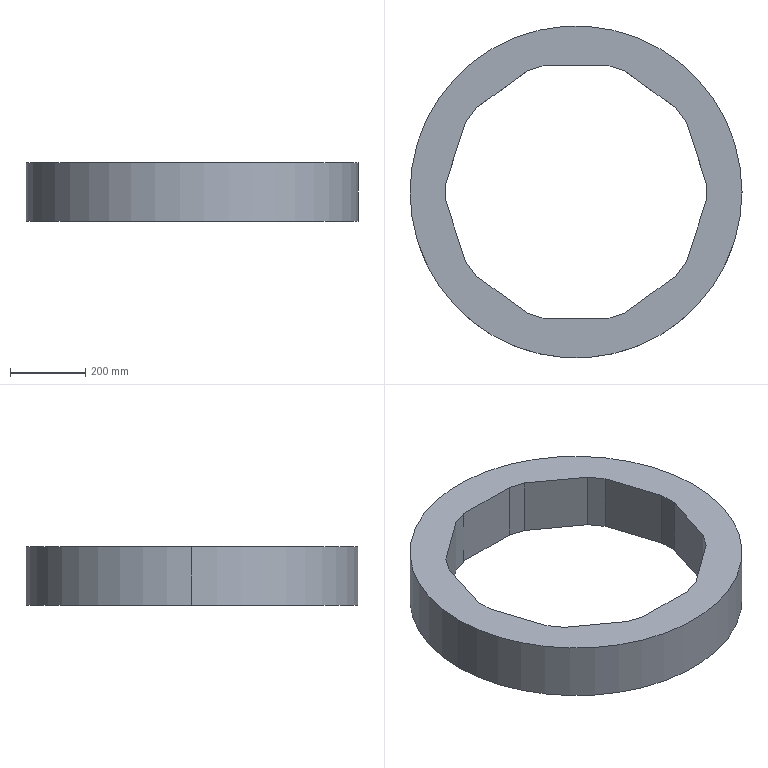Part | SolidWorks | features Extrusion 1 | 1 solid | 24 faces | box 884 x 884 x 155 mm | volume 38209027 mm3 | plane 22 | cylinder 2 | commonest cylinder face diameters 884 x2
STEP:
#1=CARTESIAN_POINT('',(442.,0.,77.5));
#2=VERTEX_POINT('',#1);
#3=CARTESIAN_POINT('',(-442.,0.,77.5));
#4=VERTEX_POINT('',#3);
#5=CARTESIAN_POINT('',(0.,0.,77.5));
#6=DIRECTION('',(0.,0.,1.));
#7=DIRECTION('',(1.,0.,0.));
#8=AXIS2_PLACEMENT_3D('',#5,#6,#7);
#9=CIRCLE('',#8,442.);
#10=EDGE_CURVE('',#2,#4,#9,.T.);
#11=ORIENTED_EDGE('',*,*,#10,.F.);
#12=CARTESIAN_POINT('',(442.,0.,-77.5));
#13=VERTEX_POINT('',#12);
#14=CARTESIAN_POINT('',(442.,0.,77.5));
#15=DIRECTION('',(0.,0.,-1.));
#16=VECTOR('',#15,1000.);
#17=LINE('',#14,#16);
#18=EDGE_CURVE('',#2,#13,#17,.T.);
#19=ORIENTED_EDGE('',*,*,#18,.T.);
#20=CARTESIAN_POINT('',(-442.,0.,-77.5));
#21=VERTEX_POINT('',#20);
#22=CARTESIAN_POINT('',(0.,0.,-77.5));
#23=DIRECTION('',(0.,0.,1.));
#24=DIRECTION('',(1.,0.,0.));
#25=AXIS2_PLACEMENT_3D('',#22,#23,#24);
#26=CIRCLE('',#25,442.);
#27=EDGE_CURVE('',#13,#21,#26,.T.);
#28=ORIENTED_EDGE('',*,*,#27,.T.);
#29=CARTESIAN_POINT('',(-442.,0.,77.5));
#30=DIRECTION('',(0.,0.,-1.));
#31=VECTOR('',#30,1000.);
#32=LINE('',#29,#31);
#33=EDGE_CURVE('',#4,#21,#32,.T.);
#34=ORIENTED_EDGE('',*,*,#33,.F.);
#35=EDGE_LOOP('',(#11,#19,#28,#34));
#36=FACE_OUTER_BOUND('',#35,.T.);
#37=CARTESIAN_POINT('',(0.,0.,77.5));
#38=DIRECTION('',(0.,0.,-1.));
#39=DIRECTION('',(-1.,0.,0.));
#40=AXIS2_PLACEMENT_3D('',#37,#38,#39);
#41=CYLINDRICAL_SURFACE('',#40,442.);
#42=ADVANCED_FACE('',(#36),#41,.T.);
#43=CARTESIAN_POINT('',(0.,0.,77.5));
#44=DIRECTION('',(0.,0.,1.));
#45=DIRECTION('',(1.,0.,0.));
#46=AXIS2_PLACEMENT_3D('',#43,#44,#45);
#47=CIRCLE('',#46,442.);
#48=EDGE_CURVE('',#4,#2,#47,.T.);
#49=ORIENTED_EDGE('',*,*,#48,.T.);
#50=ORIENTED_EDGE('',*,*,#10,.T.);
#51=EDGE_LOOP('',(#49,#50));
#52=FACE_OUTER_BOUND('',#51,.T.);
#53=CARTESIAN_POINT('',(346.772,-23.299,77.5));
#54=VERTEX_POINT('',#53);
#55=CARTESIAN_POINT('',(346.772,23.299,77.5));
#56=VERTEX_POINT('',#55);
#57=CARTESIAN_POINT('',(346.772,-23.299,77.5));
#58=DIRECTION('',(0.,1.,0.));
#59=VECTOR('',#58,1000.);
#60=LINE('',#57,#59);
#61=EDGE_CURVE('',#54,#56,#60,.T.);
#62=ORIENTED_EDGE('',*,*,#61,.F.);
#63=CARTESIAN_POINT('',(294.24,-184.979,77.5));
#64=VERTEX_POINT('',#63);
#65=CARTESIAN_POINT('',(346.772,-23.299,77.5));
#66=DIRECTION('',(0.309,0.9511,0.));
#67=VECTOR('',#66,1000.);
#68=LINE('',#65,#67);
#69=EDGE_CURVE('',#64,#54,#68,.T.);
#70=ORIENTED_EDGE('',*,*,#69,.F.);
#71=CARTESIAN_POINT('',(266.85,-222.677,77.5));
#72=VERTEX_POINT('',#71);
#73=CARTESIAN_POINT('',(294.24,-184.979,77.5));
#74=DIRECTION('',(0.5878,0.809,0.));
#75=VECTOR('',#74,1000.);
#76=LINE('',#73,#75);
#77=EDGE_CURVE('',#72,#64,#76,.T.);
#78=ORIENTED_EDGE('',*,*,#77,.F.);
#79=CARTESIAN_POINT('',(129.317,-322.6,77.5));
#80=VERTEX_POINT('',#79);
#81=CARTESIAN_POINT('',(266.85,-222.677,77.5));
#82=DIRECTION('',(0.809,0.5878,0.));
#83=VECTOR('',#82,1000.);
#84=LINE('',#81,#83);
#85=EDGE_CURVE('',#80,#72,#84,.T.);
#86=ORIENTED_EDGE('',*,*,#85,.F.);
#87=CARTESIAN_POINT('',(85.,-337.,77.5));
#88=VERTEX_POINT('',#87);
#89=CARTESIAN_POINT('',(85.,-337.,77.5));
#90=DIRECTION('',(0.9511,0.309,0.));
#91=VECTOR('',#90,1000.);
#92=LINE('',#89,#91);
#93=EDGE_CURVE('',#88,#80,#92,.T.);
#94=ORIENTED_EDGE('',*,*,#93,.F.);
#95=CARTESIAN_POINT('',(-85.,-337.,77.5));
#96=VERTEX_POINT('',#95);
#97=CARTESIAN_POINT('',(85.,-337.,77.5));
#98=DIRECTION('',(1.,0.,0.));
#99=VECTOR('',#98,1000.);
#100=LINE('',#97,#99);
#101=EDGE_CURVE('',#96,#88,#100,.T.);
#102=ORIENTED_EDGE('',*,*,#101,.F.);
#103=CARTESIAN_POINT('',(-129.317,-322.6,77.5));
#104=VERTEX_POINT('',#103);
#105=CARTESIAN_POINT('',(-129.317,-322.6,77.5));
#106=DIRECTION('',(0.9511,-0.309,0.));
#107=VECTOR('',#106,1000.);
#108=LINE('',#105,#107);
#109=EDGE_CURVE('',#104,#96,#108,.T.);
#110=ORIENTED_EDGE('',*,*,#109,.F.);
#111=CARTESIAN_POINT('',(-266.85,-222.677,77.5));
#112=VERTEX_POINT('',#111);
#113=CARTESIAN_POINT('',(-129.317,-322.6,77.5));
#114=DIRECTION('',(0.809,-0.5878,0.));
#115=VECTOR('',#114,1000.);
#116=LINE('',#113,#115);
#117=EDGE_CURVE('',#112,#104,#116,.T.);
#118=ORIENTED_EDGE('',*,*,#117,.F.);
#119=CARTESIAN_POINT('',(-294.24,-184.979,77.5));
#120=VERTEX_POINT('',#119);
#121=CARTESIAN_POINT('',(-294.24,-184.979,77.5));
#122=DIRECTION('',(0.5878,-0.809,0.));
#123=VECTOR('',#122,1000.);
#124=LINE('',#121,#123);
#125=EDGE_CURVE('',#120,#112,#124,.T.);
#126=ORIENTED_EDGE('',*,*,#125,.F.);
#127=CARTESIAN_POINT('',(-346.772,-23.299,77.5));
#128=VERTEX_POINT('',#127);
#129=CARTESIAN_POINT('',(-294.24,-184.979,77.5));
#130=DIRECTION('',(0.309,-0.9511,0.));
#131=VECTOR('',#130,1000.);
#132=LINE('',#129,#131);
#133=EDGE_CURVE('',#128,#120,#132,.T.);
#134=ORIENTED_EDGE('',*,*,#133,.F.);
#135=CARTESIAN_POINT('',(-346.772,23.299,77.5));
#136=VERTEX_POINT('',#135);
#137=CARTESIAN_POINT('',(-346.772,23.299,77.5));
#138=DIRECTION('',(0.,-1.,0.));
#139=VECTOR('',#138,1000.);
#140=LINE('',#137,#139);
#141=EDGE_CURVE('',#136,#128,#140,.T.);
#142=ORIENTED_EDGE('',*,*,#141,.F.);
#143=CARTESIAN_POINT('',(-294.24,184.979,77.5));
#144=VERTEX_POINT('',#143);
#145=CARTESIAN_POINT('',(-346.772,23.299,77.5));
#146=DIRECTION('',(-0.309,-0.9511,0.));
#147=VECTOR('',#146,1000.);
#148=LINE('',#145,#147);
#149=EDGE_CURVE('',#144,#136,#148,.T.);
#150=ORIENTED_EDGE('',*,*,#149,.F.);
#151=CARTESIAN_POINT('',(-266.85,222.677,77.5));
#152=VERTEX_POINT('',#151);
#153=CARTESIAN_POINT('',(-266.85,222.677,77.5));
#154=DIRECTION('',(-0.5878,-0.809,0.));
#155=VECTOR('',#154,1000.);
#156=LINE('',#153,#155);
#157=EDGE_CURVE('',#152,#144,#156,.T.);
#158=ORIENTED_EDGE('',*,*,#157,.F.);
#159=CARTESIAN_POINT('',(-129.317,322.6,77.5));
#160=VERTEX_POINT('',#159);
#161=CARTESIAN_POINT('',(-266.85,222.677,77.5));
#162=DIRECTION('',(-0.809,-0.5878,0.));
#163=VECTOR('',#162,1000.);
#164=LINE('',#161,#163);
#165=EDGE_CURVE('',#160,#152,#164,.T.);
#166=ORIENTED_EDGE('',*,*,#165,.F.);
#167=CARTESIAN_POINT('',(-85.,337.,77.5));
#168=VERTEX_POINT('',#167);
#169=CARTESIAN_POINT('',(-85.,337.,77.5));
#170=DIRECTION('',(-0.9511,-0.309,0.));
#171=VECTOR('',#170,1000.);
#172=LINE('',#169,#171);
#173=EDGE_CURVE('',#168,#160,#172,.T.);
#174=ORIENTED_EDGE('',*,*,#173,.F.);
#175=CARTESIAN_POINT('',(85.,337.,77.5));
#176=VERTEX_POINT('',#175);
#177=CARTESIAN_POINT('',(-85.,337.,77.5));
#178=DIRECTION('',(-1.,0.,0.));
#179=VECTOR('',#178,1000.);
#180=LINE('',#177,#179);
#181=EDGE_CURVE('',#176,#168,#180,.T.);
#182=ORIENTED_EDGE('',*,*,#181,.F.);
#183=CARTESIAN_POINT('',(129.317,322.6,77.5));
#184=VERTEX_POINT('',#183);
#185=CARTESIAN_POINT('',(129.317,322.6,77.5));
#186=DIRECTION('',(-0.9511,0.309,0.));
#187=VECTOR('',#186,1000.);
#188=LINE('',#185,#187);
#189=EDGE_CURVE('',#184,#176,#188,.T.);
#190=ORIENTED_EDGE('',*,*,#189,.F.);
#191=CARTESIAN_POINT('',(266.85,222.677,77.5));
#192=VERTEX_POINT('',#191);
#193=CARTESIAN_POINT('',(129.317,322.6,77.5));
#194=DIRECTION('',(-0.809,0.5878,0.));
#195=VECTOR('',#194,1000.);
#196=LINE('',#193,#195);
#197=EDGE_CURVE('',#192,#184,#196,.T.);
#198=ORIENTED_EDGE('',*,*,#197,.F.);
#199=CARTESIAN_POINT('',(294.24,184.979,77.5));
#200=VERTEX_POINT('',#199);
#201=CARTESIAN_POINT('',(294.24,184.979,77.5));
#202=DIRECTION('',(-0.5878,0.809,0.));
#203=VECTOR('',#202,1000.);
#204=LINE('',#201,#203);
#205=EDGE_CURVE('',#200,#192,#204,.T.);
#206=ORIENTED_EDGE('',*,*,#205,.F.);
#207=CARTESIAN_POINT('',(294.24,184.979,77.5));
#208=DIRECTION('',(-0.309,0.9511,0.));
#209=VECTOR('',#208,1000.);
#210=LINE('',#207,#209);
#211=EDGE_CURVE('',#56,#200,#210,.T.);
#212=ORIENTED_EDGE('',*,*,#211,.F.);
#213=EDGE_LOOP('',(#62,#70,#78,#86,#94,#102,#110,#118,#126,#134,#142,#150,#158,#166,#174,#182,#190,#198,#206,#212));
#214=FACE_BOUND('',#213,.T.);
#215=CARTESIAN_POINT('',(0.,0.,77.5));
#216=DIRECTION('',(0.,0.,1.));
#217=DIRECTION('',(1.,0.,0.));
#218=AXIS2_PLACEMENT_3D('',#215,#216,#217);
#219=PLANE('',#218);
#220=ADVANCED_FACE('',(#52,#214),#219,.T.);
#221=CARTESIAN_POINT('',(0.,0.,-77.5));
#222=DIRECTION('',(0.,0.,1.));
#223=DIRECTION('',(1.,0.,0.));
#224=AXIS2_PLACEMENT_3D('',#221,#222,#223);
#225=CIRCLE('',#224,442.);
#226=EDGE_CURVE('',#21,#13,#225,.T.);
#227=ORIENTED_EDGE('',*,*,#226,.F.);
#228=ORIENTED_EDGE('',*,*,#27,.F.);
#229=EDGE_LOOP('',(#227,#228));
#230=FACE_OUTER_BOUND('',#229,.T.);
#231=CARTESIAN_POINT('',(294.24,-184.979,-77.5));
#232=VERTEX_POINT('',#231);
#233=CARTESIAN_POINT('',(346.772,-23.299,-77.5));
#234=VERTEX_POINT('',#233);
#235=CARTESIAN_POINT('',(346.772,-23.299,-77.5));
#236=DIRECTION('',(0.309,0.9511,0.));
#237=VECTOR('',#236,1000.);
#238=LINE('',#235,#237);
#239=EDGE_CURVE('',#232,#234,#238,.T.);
#240=ORIENTED_EDGE('',*,*,#239,.T.);
#241=CARTESIAN_POINT('',(346.772,23.299,-77.5));
#242=VERTEX_POINT('',#241);
#243=CARTESIAN_POINT('',(346.772,-23.299,-77.5));
#244=DIRECTION('',(0.,1.,0.));
#245=VECTOR('',#244,1000.);
#246=LINE('',#243,#245);
#247=EDGE_CURVE('',#234,#242,#246,.T.);
#248=ORIENTED_EDGE('',*,*,#247,.T.);
#249=CARTESIAN_POINT('',(294.24,184.979,-77.5));
#250=VERTEX_POINT('',#249);
#251=CARTESIAN_POINT('',(294.24,184.979,-77.5));
#252=DIRECTION('',(-0.309,0.9511,0.));
#253=VECTOR('',#252,1000.);
#254=LINE('',#251,#253);
#255=EDGE_CURVE('',#242,#250,#254,.T.);
#256=ORIENTED_EDGE('',*,*,#255,.T.);
#257=CARTESIAN_POINT('',(266.85,222.677,-77.5));
#258=VERTEX_POINT('',#257);
#259=CARTESIAN_POINT('',(294.24,184.979,-77.5));
#260=DIRECTION('',(-0.5878,0.809,0.));
#261=VECTOR('',#260,1000.);
#262=LINE('',#259,#261);
#263=EDGE_CURVE('',#250,#258,#262,.T.);
#264=ORIENTED_EDGE('',*,*,#263,.T.);
#265=CARTESIAN_POINT('',(129.317,322.6,-77.5));
#266=VERTEX_POINT('',#265);
#267=CARTESIAN_POINT('',(129.317,322.6,-77.5));
#268=DIRECTION('',(-0.809,0.5878,0.));
#269=VECTOR('',#268,1000.);
#270=LINE('',#267,#269);
#271=EDGE_CURVE('',#258,#266,#270,.T.);
#272=ORIENTED_EDGE('',*,*,#271,.T.);
#273=CARTESIAN_POINT('',(85.,337.,-77.5));
#274=VERTEX_POINT('',#273);
#275=CARTESIAN_POINT('',(129.317,322.6,-77.5));
#276=DIRECTION('',(-0.9511,0.309,0.));
#277=VECTOR('',#276,1000.);
#278=LINE('',#275,#277);
#279=EDGE_CURVE('',#266,#274,#278,.T.);
#280=ORIENTED_EDGE('',*,*,#279,.T.);
#281=CARTESIAN_POINT('',(-85.,337.,-77.5));
#282=VERTEX_POINT('',#281);
#283=CARTESIAN_POINT('',(-85.,337.,-77.5));
#284=DIRECTION('',(-1.,0.,0.));
#285=VECTOR('',#284,1000.);
#286=LINE('',#283,#285);
#287=EDGE_CURVE('',#274,#282,#286,.T.);
#288=ORIENTED_EDGE('',*,*,#287,.T.);
#289=CARTESIAN_POINT('',(-129.317,322.6,-77.5));
#290=VERTEX_POINT('',#289);
#291=CARTESIAN_POINT('',(-85.,337.,-77.5));
#292=DIRECTION('',(-0.9511,-0.309,0.));
#293=VECTOR('',#292,1000.);
#294=LINE('',#291,#293);
#295=EDGE_CURVE('',#282,#290,#294,.T.);
#296=ORIENTED_EDGE('',*,*,#295,.T.);
#297=CARTESIAN_POINT('',(-266.85,222.677,-77.5));
#298=VERTEX_POINT('',#297);
#299=CARTESIAN_POINT('',(-266.85,222.677,-77.5));
#300=DIRECTION('',(-0.809,-0.5878,0.));
#301=VECTOR('',#300,1000.);
#302=LINE('',#299,#301);
#303=EDGE_CURVE('',#290,#298,#302,.T.);
#304=ORIENTED_EDGE('',*,*,#303,.T.);
#305=CARTESIAN_POINT('',(-294.24,184.979,-77.5));
#306=VERTEX_POINT('',#305);
#307=CARTESIAN_POINT('',(-266.85,222.677,-77.5));
#308=DIRECTION('',(-0.5878,-0.809,0.));
#309=VECTOR('',#308,1000.);
#310=LINE('',#307,#309);
#311=EDGE_CURVE('',#298,#306,#310,.T.);
#312=ORIENTED_EDGE('',*,*,#311,.T.);
#313=CARTESIAN_POINT('',(-346.772,23.299,-77.5));
#314=VERTEX_POINT('',#313);
#315=CARTESIAN_POINT('',(-346.772,23.299,-77.5));
#316=DIRECTION('',(-0.309,-0.9511,0.));
#317=VECTOR('',#316,1000.);
#318=LINE('',#315,#317);
#319=EDGE_CURVE('',#306,#314,#318,.T.);
#320=ORIENTED_EDGE('',*,*,#319,.T.);
#321=CARTESIAN_POINT('',(-346.772,-23.299,-77.5));
#322=VERTEX_POINT('',#321);
#323=CARTESIAN_POINT('',(-346.772,23.299,-77.5));
#324=DIRECTION('',(0.,-1.,0.));
#325=VECTOR('',#324,1000.);
#326=LINE('',#323,#325);
#327=EDGE_CURVE('',#314,#322,#326,.T.);
#328=ORIENTED_EDGE('',*,*,#327,.T.);
#329=CARTESIAN_POINT('',(-294.24,-184.979,-77.5));
#330=VERTEX_POINT('',#329);
#331=CARTESIAN_POINT('',(-294.24,-184.979,-77.5));
#332=DIRECTION('',(0.309,-0.9511,0.));
#333=VECTOR('',#332,1000.);
#334=LINE('',#331,#333);
#335=EDGE_CURVE('',#322,#330,#334,.T.);
#336=ORIENTED_EDGE('',*,*,#335,.T.);
#337=CARTESIAN_POINT('',(-266.85,-222.677,-77.5));
#338=VERTEX_POINT('',#337);
#339=CARTESIAN_POINT('',(-294.24,-184.979,-77.5));
#340=DIRECTION('',(0.5878,-0.809,0.));
#341=VECTOR('',#340,1000.);
#342=LINE('',#339,#341);
#343=EDGE_CURVE('',#330,#338,#342,.T.);
#344=ORIENTED_EDGE('',*,*,#343,.T.);
#345=CARTESIAN_POINT('',(-129.317,-322.6,-77.5));
#346=VERTEX_POINT('',#345);
#347=CARTESIAN_POINT('',(-129.317,-322.6,-77.5));
#348=DIRECTION('',(0.809,-0.5878,0.));
#349=VECTOR('',#348,1000.);
#350=LINE('',#347,#349);
#351=EDGE_CURVE('',#338,#346,#350,.T.);
#352=ORIENTED_EDGE('',*,*,#351,.T.);
#353=CARTESIAN_POINT('',(-85.,-337.,-77.5));
#354=VERTEX_POINT('',#353);
#355=CARTESIAN_POINT('',(-129.317,-322.6,-77.5));
#356=DIRECTION('',(0.9511,-0.309,0.));
#357=VECTOR('',#356,1000.);
#358=LINE('',#355,#357);
#359=EDGE_CURVE('',#346,#354,#358,.T.);
#360=ORIENTED_EDGE('',*,*,#359,.T.);
#361=CARTESIAN_POINT('',(85.,-337.,-77.5));
#362=VERTEX_POINT('',#361);
#363=CARTESIAN_POINT('',(85.,-337.,-77.5));
#364=DIRECTION('',(1.,0.,0.));
#365=VECTOR('',#364,1000.);
#366=LINE('',#363,#365);
#367=EDGE_CURVE('',#354,#362,#366,.T.);
#368=ORIENTED_EDGE('',*,*,#367,.T.);
#369=CARTESIAN_POINT('',(129.317,-322.6,-77.5));
#370=VERTEX_POINT('',#369);
#371=CARTESIAN_POINT('',(85.,-337.,-77.5));
#372=DIRECTION('',(0.9511,0.309,0.));
#373=VECTOR('',#372,1000.);
#374=LINE('',#371,#373);
#375=EDGE_CURVE('',#362,#370,#374,.T.);
#376=ORIENTED_EDGE('',*,*,#375,.T.);
#377=CARTESIAN_POINT('',(266.85,-222.677,-77.5));
#378=VERTEX_POINT('',#377);
#379=CARTESIAN_POINT('',(266.85,-222.677,-77.5));
#380=DIRECTION('',(0.809,0.5878,0.));
#381=VECTOR('',#380,1000.);
#382=LINE('',#379,#381);
#383=EDGE_CURVE('',#370,#378,#382,.T.);
#384=ORIENTED_EDGE('',*,*,#383,.T.);
#385=CARTESIAN_POINT('',(294.24,-184.979,-77.5));
#386=DIRECTION('',(0.5878,0.809,0.));
#387=VECTOR('',#386,1000.);
#388=LINE('',#385,#387);
#389=EDGE_CURVE('',#378,#232,#388,.T.);
#390=ORIENTED_EDGE('',*,*,#389,.T.);
#391=EDGE_LOOP('',(#240,#248,#256,#264,#272,#280,#288,#296,#304,#312,#320,#328,#336,#344,#352,#360,#368,#376,#384,#390));
#392=FACE_BOUND('',#391,.T.);
#393=CARTESIAN_POINT('',(0.,0.,-77.5));
#394=DIRECTION('',(0.,0.,1.));
#395=DIRECTION('',(1.,0.,0.));
#396=AXIS2_PLACEMENT_3D('',#393,#394,#395);
#397=PLANE('',#396);
#398=ADVANCED_FACE('',(#230,#392),#397,.F.);
#399=ORIENTED_EDGE('',*,*,#18,.F.);
#400=ORIENTED_EDGE('',*,*,#48,.F.);
#401=ORIENTED_EDGE('',*,*,#33,.T.);
#402=ORIENTED_EDGE('',*,*,#226,.T.);
#403=EDGE_LOOP('',(#399,#400,#401,#402));
#404=FACE_OUTER_BOUND('',#403,.T.);
#405=CARTESIAN_POINT('',(0.,0.,77.5));
#406=DIRECTION('',(0.,0.,-1.));
#407=DIRECTION('',(-1.,0.,0.));
#408=AXIS2_PLACEMENT_3D('',#405,#406,#407);
#409=CYLINDRICAL_SURFACE('',#408,442.);
#410=ADVANCED_FACE('',(#404),#409,.T.);
#411=ORIENTED_EDGE('',*,*,#239,.F.);
#412=CARTESIAN_POINT('',(294.24,-184.979,77.5));
#413=DIRECTION('',(0.,0.,-1.));
#414=VECTOR('',#413,1000.);
#415=LINE('',#412,#414);
#416=EDGE_CURVE('',#64,#232,#415,.T.);
#417=ORIENTED_EDGE('',*,*,#416,.F.);
#418=ORIENTED_EDGE('',*,*,#69,.T.);
#419=CARTESIAN_POINT('',(346.772,-23.299,77.5));
#420=DIRECTION('',(0.,0.,-1.));
#421=VECTOR('',#420,1000.);
#422=LINE('',#419,#421);
#423=EDGE_CURVE('',#54,#234,#422,.T.);
#424=ORIENTED_EDGE('',*,*,#423,.T.);
#425=EDGE_LOOP('',(#411,#417,#418,#424));
#426=FACE_OUTER_BOUND('',#425,.T.);
#427=CARTESIAN_POINT('',(346.772,-23.299,77.5));
#428=DIRECTION('',(-0.9511,0.309,0.));
#429=DIRECTION('',(-0.309,-0.9511,0.));
#430=AXIS2_PLACEMENT_3D('',#427,#428,#429);
#431=PLANE('',#430);
#432=ADVANCED_FACE('',(#426),#431,.T.);
#433=ORIENTED_EDGE('',*,*,#247,.F.);
#434=ORIENTED_EDGE('',*,*,#423,.F.);
#435=ORIENTED_EDGE('',*,*,#61,.T.);
#436=CARTESIAN_POINT('',(346.772,23.299,77.5));
#437=DIRECTION('',(0.,0.,-1.));
#438=VECTOR('',#437,1000.);
#439=LINE('',#436,#438);
#440=EDGE_CURVE('',#56,#242,#439,.T.);
#441=ORIENTED_EDGE('',*,*,#440,.T.);
#442=EDGE_LOOP('',(#433,#434,#435,#441));
#443=FACE_OUTER_BOUND('',#442,.T.);
#444=CARTESIAN_POINT('',(346.772,-23.299,77.5));
#445=DIRECTION('',(-1.,0.,0.));
#446=DIRECTION('',(0.,-1.,0.));
#447=AXIS2_PLACEMENT_3D('',#444,#445,#446);
#448=PLANE('',#447);
#449=ADVANCED_FACE('',(#443),#448,.T.);
#450=ORIENTED_EDGE('',*,*,#255,.F.);
#451=ORIENTED_EDGE('',*,*,#440,.F.);
#452=ORIENTED_EDGE('',*,*,#211,.T.);
#453=CARTESIAN_POINT('',(294.24,184.979,77.5));
#454=DIRECTION('',(0.,0.,-1.));
#455=VECTOR('',#454,1000.);
#456=LINE('',#453,#455);
#457=EDGE_CURVE('',#200,#250,#456,.T.);
#458=ORIENTED_EDGE('',*,*,#457,.T.);
#459=EDGE_LOOP('',(#450,#451,#452,#458));
#460=FACE_OUTER_BOUND('',#459,.T.);
#461=CARTESIAN_POINT('',(294.24,184.979,77.5));
#462=DIRECTION('',(-0.9511,-0.309,0.));
#463=DIRECTION('',(0.309,-0.9511,0.));
#464=AXIS2_PLACEMENT_3D('',#461,#462,#463);
#465=PLANE('',#464);
#466=ADVANCED_FACE('',(#460),#465,.T.);
#467=ORIENTED_EDGE('',*,*,#263,.F.);
#468=ORIENTED_EDGE('',*,*,#457,.F.);
#469=ORIENTED_EDGE('',*,*,#205,.T.);
#470=CARTESIAN_POINT('',(266.85,222.677,77.5));
#471=DIRECTION('',(0.,0.,-1.));
#472=VECTOR('',#471,1000.);
#473=LINE('',#470,#472);
#474=EDGE_CURVE('',#192,#258,#473,.T.);
#475=ORIENTED_EDGE('',*,*,#474,.T.);
#476=EDGE_LOOP('',(#467,#468,#469,#475));
#477=FACE_OUTER_BOUND('',#476,.T.);
#478=CARTESIAN_POINT('',(294.24,184.979,77.5));
#479=DIRECTION('',(-0.809,-0.5878,0.));
#480=DIRECTION('',(0.5878,-0.809,0.));
#481=AXIS2_PLACEMENT_3D('',#478,#479,#480);
#482=PLANE('',#481);
#483=ADVANCED_FACE('',(#477),#482,.T.);
#484=ORIENTED_EDGE('',*,*,#271,.F.);
#485=ORIENTED_EDGE('',*,*,#474,.F.);
#486=ORIENTED_EDGE('',*,*,#197,.T.);
#487=CARTESIAN_POINT('',(129.317,322.6,77.5));
#488=DIRECTION('',(0.,0.,-1.));
#489=VECTOR('',#488,1000.);
#490=LINE('',#487,#489);
#491=EDGE_CURVE('',#184,#266,#490,.T.);
#492=ORIENTED_EDGE('',*,*,#491,.T.);
#493=EDGE_LOOP('',(#484,#485,#486,#492));
#494=FACE_OUTER_BOUND('',#493,.T.);
#495=CARTESIAN_POINT('',(129.317,322.6,77.5));
#496=DIRECTION('',(-0.5878,-0.809,0.));
#497=DIRECTION('',(0.809,-0.5878,0.));
#498=AXIS2_PLACEMENT_3D('',#495,#496,#497);
#499=PLANE('',#498);
#500=ADVANCED_FACE('',(#494),#499,.T.);
#501=ORIENTED_EDGE('',*,*,#279,.F.);
#502=ORIENTED_EDGE('',*,*,#491,.F.);
#503=ORIENTED_EDGE('',*,*,#189,.T.);
#504=CARTESIAN_POINT('',(85.,337.,77.5));
#505=DIRECTION('',(0.,0.,-1.));
#506=VECTOR('',#505,1000.);
#507=LINE('',#504,#506);
#508=EDGE_CURVE('',#176,#274,#507,.T.);
#509=ORIENTED_EDGE('',*,*,#508,.T.);
#510=EDGE_LOOP('',(#501,#502,#503,#509));
#511=FACE_OUTER_BOUND('',#510,.T.);
#512=CARTESIAN_POINT('',(129.317,322.6,77.5));
#513=DIRECTION('',(-0.309,-0.9511,0.));
#514=DIRECTION('',(0.9511,-0.309,0.));
#515=AXIS2_PLACEMENT_3D('',#512,#513,#514);
#516=PLANE('',#515);
#517=ADVANCED_FACE('',(#511),#516,.T.);
#518=ORIENTED_EDGE('',*,*,#287,.F.);
#519=ORIENTED_EDGE('',*,*,#508,.F.);
#520=ORIENTED_EDGE('',*,*,#181,.T.);
#521=CARTESIAN_POINT('',(-85.,337.,77.5));
#522=DIRECTION('',(0.,0.,-1.));
#523=VECTOR('',#522,1000.);
#524=LINE('',#521,#523);
#525=EDGE_CURVE('',#168,#282,#524,.T.);
#526=ORIENTED_EDGE('',*,*,#525,.T.);
#527=EDGE_LOOP('',(#518,#519,#520,#526));
#528=FACE_OUTER_BOUND('',#527,.T.);
#529=CARTESIAN_POINT('',(-85.,337.,77.5));
#530=DIRECTION('',(0.,-1.,0.));
#531=DIRECTION('',(1.,0.,0.));
#532=AXIS2_PLACEMENT_3D('',#529,#530,#531);
#533=PLANE('',#532);
#534=ADVANCED_FACE('',(#528),#533,.T.);
#535=ORIENTED_EDGE('',*,*,#295,.F.);
#536=ORIENTED_EDGE('',*,*,#525,.F.);
#537=ORIENTED_EDGE('',*,*,#173,.T.);
#538=CARTESIAN_POINT('',(-129.317,322.6,77.5));
#539=DIRECTION('',(0.,0.,-1.));
#540=VECTOR('',#539,1000.);
#541=LINE('',#538,#540);
#542=EDGE_CURVE('',#160,#290,#541,.T.);
#543=ORIENTED_EDGE('',*,*,#542,.T.);
#544=EDGE_LOOP('',(#535,#536,#537,#543));
#545=FACE_OUTER_BOUND('',#544,.T.);
#546=CARTESIAN_POINT('',(-85.,337.,77.5));
#547=DIRECTION('',(0.309,-0.9511,0.));
#548=DIRECTION('',(0.9511,0.309,0.));
#549=AXIS2_PLACEMENT_3D('',#546,#547,#548);
#550=PLANE('',#549);
#551=ADVANCED_FACE('',(#545),#550,.T.);
#552=ORIENTED_EDGE('',*,*,#303,.F.);
#553=ORIENTED_EDGE('',*,*,#542,.F.);
#554=ORIENTED_EDGE('',*,*,#165,.T.);
#555=CARTESIAN_POINT('',(-266.85,222.677,77.5));
#556=DIRECTION('',(0.,0.,-1.));
#557=VECTOR('',#556,1000.);
#558=LINE('',#555,#557);
#559=EDGE_CURVE('',#152,#298,#558,.T.);
#560=ORIENTED_EDGE('',*,*,#559,.T.);
#561=EDGE_LOOP('',(#552,#553,#554,#560));
#562=FACE_OUTER_BOUND('',#561,.T.);
#563=CARTESIAN_POINT('',(-266.85,222.677,77.5));
#564=DIRECTION('',(0.5878,-0.809,0.));
#565=DIRECTION('',(0.809,0.5878,0.));
#566=AXIS2_PLACEMENT_3D('',#563,#564,#565);
#567=PLANE('',#566);
#568=ADVANCED_FACE('',(#562),#567,.T.);
#569=ORIENTED_EDGE('',*,*,#311,.F.);
#570=ORIENTED_EDGE('',*,*,#559,.F.);
#571=ORIENTED_EDGE('',*,*,#157,.T.);
#572=CARTESIAN_POINT('',(-294.24,184.979,77.5));
#573=DIRECTION('',(0.,0.,-1.));
#574=VECTOR('',#573,1000.);
#575=LINE('',#572,#574);
#576=EDGE_CURVE('',#144,#306,#575,.T.);
#577=ORIENTED_EDGE('',*,*,#576,.T.);
#578=EDGE_LOOP('',(#569,#570,#571,#577));
#579=FACE_OUTER_BOUND('',#578,.T.);
#580=CARTESIAN_POINT('',(-266.85,222.677,77.5));
#581=DIRECTION('',(0.809,-0.5878,0.));
#582=DIRECTION('',(0.5878,0.809,0.));
#583=AXIS2_PLACEMENT_3D('',#580,#581,#582);
#584=PLANE('',#583);
#585=ADVANCED_FACE('',(#579),#584,.T.);
#586=ORIENTED_EDGE('',*,*,#319,.F.);
#587=ORIENTED_EDGE('',*,*,#576,.F.);
#588=ORIENTED_EDGE('',*,*,#149,.T.);
#589=CARTESIAN_POINT('',(-346.772,23.299,77.5));
#590=DIRECTION('',(0.,0.,-1.));
#591=VECTOR('',#590,1000.);
#592=LINE('',#589,#591);
#593=EDGE_CURVE('',#136,#314,#592,.T.);
#594=ORIENTED_EDGE('',*,*,#593,.T.);
#595=EDGE_LOOP('',(#586,#587,#588,#594));
#596=FACE_OUTER_BOUND('',#595,.T.);
#597=CARTESIAN_POINT('',(-346.772,23.299,77.5));
#598=DIRECTION('',(0.9511,-0.309,0.));
#599=DIRECTION('',(0.309,0.9511,0.));
#600=AXIS2_PLACEMENT_3D('',#597,#598,#599);
#601=PLANE('',#600);
#602=ADVANCED_FACE('',(#596),#601,.T.);
#603=ORIENTED_EDGE('',*,*,#327,.F.);
#604=ORIENTED_EDGE('',*,*,#593,.F.);
#605=ORIENTED_EDGE('',*,*,#141,.T.);
#606=CARTESIAN_POINT('',(-346.772,-23.299,77.5));
#607=DIRECTION('',(0.,0.,-1.));
#608=VECTOR('',#607,1000.);
#609=LINE('',#606,#608);
#610=EDGE_CURVE('',#128,#322,#609,.T.);
#611=ORIENTED_EDGE('',*,*,#610,.T.);
#612=EDGE_LOOP('',(#603,#604,#605,#611));
#613=FACE_OUTER_BOUND('',#612,.T.);
#614=CARTESIAN_POINT('',(-346.772,23.299,77.5));
#615=DIRECTION('',(1.,0.,0.));
#616=DIRECTION('',(0.,1.,0.));
#617=AXIS2_PLACEMENT_3D('',#614,#615,#616);
#618=PLANE('',#617);
#619=ADVANCED_FACE('',(#613),#618,.T.);
#620=ORIENTED_EDGE('',*,*,#335,.F.);
#621=ORIENTED_EDGE('',*,*,#610,.F.);
#622=ORIENTED_EDGE('',*,*,#133,.T.);
#623=CARTESIAN_POINT('',(-294.24,-184.979,77.5));
#624=DIRECTION('',(0.,0.,-1.));
#625=VECTOR('',#624,1000.);
#626=LINE('',#623,#625);
#627=EDGE_CURVE('',#120,#330,#626,.T.);
#628=ORIENTED_EDGE('',*,*,#627,.T.);
#629=EDGE_LOOP('',(#620,#621,#622,#628));
#630=FACE_OUTER_BOUND('',#629,.T.);
#631=CARTESIAN_POINT('',(-294.24,-184.979,77.5));
#632=DIRECTION('',(0.9511,0.309,0.));
#633=DIRECTION('',(-0.309,0.9511,0.));
#634=AXIS2_PLACEMENT_3D('',#631,#632,#633);
#635=PLANE('',#634);
#636=ADVANCED_FACE('',(#630),#635,.T.);
#637=ORIENTED_EDGE('',*,*,#343,.F.);
#638=ORIENTED_EDGE('',*,*,#627,.F.);
#639=ORIENTED_EDGE('',*,*,#125,.T.);
#640=CARTESIAN_POINT('',(-266.85,-222.677,77.5));
#641=DIRECTION('',(0.,0.,-1.));
#642=VECTOR('',#641,1000.);
#643=LINE('',#640,#642);
#644=EDGE_CURVE('',#112,#338,#643,.T.);
#645=ORIENTED_EDGE('',*,*,#644,.T.);
#646=EDGE_LOOP('',(#637,#638,#639,#645));
#647=FACE_OUTER_BOUND('',#646,.T.);
#648=CARTESIAN_POINT('',(-294.24,-184.979,77.5));
#649=DIRECTION('',(0.809,0.5878,0.));
#650=DIRECTION('',(-0.5878,0.809,0.));
#651=AXIS2_PLACEMENT_3D('',#648,#649,#650);
#652=PLANE('',#651);
#653=ADVANCED_FACE('',(#647),#652,.T.);
#654=ORIENTED_EDGE('',*,*,#351,.F.);
#655=ORIENTED_EDGE('',*,*,#644,.F.);
#656=ORIENTED_EDGE('',*,*,#117,.T.);
#657=CARTESIAN_POINT('',(-129.317,-322.6,77.5));
#658=DIRECTION('',(0.,0.,-1.));
#659=VECTOR('',#658,1000.);
#660=LINE('',#657,#659);
#661=EDGE_CURVE('',#104,#346,#660,.T.);
#662=ORIENTED_EDGE('',*,*,#661,.T.);
#663=EDGE_LOOP('',(#654,#655,#656,#662));
#664=FACE_OUTER_BOUND('',#663,.T.);
#665=CARTESIAN_POINT('',(-129.317,-322.6,77.5));
#666=DIRECTION('',(0.5878,0.809,0.));
#667=DIRECTION('',(-0.809,0.5878,0.));
#668=AXIS2_PLACEMENT_3D('',#665,#666,#667);
#669=PLANE('',#668);
#670=ADVANCED_FACE('',(#664),#669,.T.);
#671=ORIENTED_EDGE('',*,*,#359,.F.);
#672=ORIENTED_EDGE('',*,*,#661,.F.);
#673=ORIENTED_EDGE('',*,*,#109,.T.);
#674=CARTESIAN_POINT('',(-85.,-337.,77.5));
#675=DIRECTION('',(0.,0.,-1.));
#676=VECTOR('',#675,1000.);
#677=LINE('',#674,#676);
#678=EDGE_CURVE('',#96,#354,#677,.T.);
#679=ORIENTED_EDGE('',*,*,#678,.T.);
#680=EDGE_LOOP('',(#671,#672,#673,#679));
#681=FACE_OUTER_BOUND('',#680,.T.);
#682=CARTESIAN_POINT('',(-129.317,-322.6,77.5));
#683=DIRECTION('',(0.309,0.9511,0.));
#684=DIRECTION('',(-0.9511,0.309,0.));
#685=AXIS2_PLACEMENT_3D('',#682,#683,#684);
#686=PLANE('',#685);
#687=ADVANCED_FACE('',(#681),#686,.T.);
#688=ORIENTED_EDGE('',*,*,#367,.F.);
#689=ORIENTED_EDGE('',*,*,#678,.F.);
#690=ORIENTED_EDGE('',*,*,#101,.T.);
#691=CARTESIAN_POINT('',(85.,-337.,77.5));
#692=DIRECTION('',(0.,0.,-1.));
#693=VECTOR('',#692,1000.);
#694=LINE('',#691,#693);
#695=EDGE_CURVE('',#88,#362,#694,.T.);
#696=ORIENTED_EDGE('',*,*,#695,.T.);
#697=EDGE_LOOP('',(#688,#689,#690,#696));
#698=FACE_OUTER_BOUND('',#697,.T.);
#699=CARTESIAN_POINT('',(85.,-337.,77.5));
#700=DIRECTION('',(0.,1.,0.));
#701=DIRECTION('',(-1.,0.,0.));
#702=AXIS2_PLACEMENT_3D('',#699,#700,#701);
#703=PLANE('',#702);
#704=ADVANCED_FACE('',(#698),#703,.T.);
#705=ORIENTED_EDGE('',*,*,#375,.F.);
#706=ORIENTED_EDGE('',*,*,#695,.F.);
#707=ORIENTED_EDGE('',*,*,#93,.T.);
#708=CARTESIAN_POINT('',(129.317,-322.6,77.5));
#709=DIRECTION('',(0.,0.,-1.));
#710=VECTOR('',#709,1000.);
#711=LINE('',#708,#710);
#712=EDGE_CURVE('',#80,#370,#711,.T.);
#713=ORIENTED_EDGE('',*,*,#712,.T.);
#714=EDGE_LOOP('',(#705,#706,#707,#713));
#715=FACE_OUTER_BOUND('',#714,.T.);
#716=CARTESIAN_POINT('',(85.,-337.,77.5));
#717=DIRECTION('',(-0.309,0.9511,0.));
#718=DIRECTION('',(-0.9511,-0.309,0.));
#719=AXIS2_PLACEMENT_3D('',#716,#717,#718);
#720=PLANE('',#719);
#721=ADVANCED_FACE('',(#715),#720,.T.);
#722=ORIENTED_EDGE('',*,*,#383,.F.);
#723=ORIENTED_EDGE('',*,*,#712,.F.);
#724=ORIENTED_EDGE('',*,*,#85,.T.);
#725=CARTESIAN_POINT('',(266.85,-222.677,77.5));
#726=DIRECTION('',(0.,0.,-1.));
#727=VECTOR('',#726,1000.);
#728=LINE('',#725,#727);
#729=EDGE_CURVE('',#72,#378,#728,.T.);
#730=ORIENTED_EDGE('',*,*,#729,.T.);
#731=EDGE_LOOP('',(#722,#723,#724,#730));
#732=FACE_OUTER_BOUND('',#731,.T.);
#733=CARTESIAN_POINT('',(266.85,-222.677,77.5));
#734=DIRECTION('',(-0.5878,0.809,0.));
#735=DIRECTION('',(-0.809,-0.5878,0.));
#736=AXIS2_PLACEMENT_3D('',#733,#734,#735);
#737=PLANE('',#736);
#738=ADVANCED_FACE('',(#732),#737,.T.);
#739=ORIENTED_EDGE('',*,*,#389,.F.);
#740=ORIENTED_EDGE('',*,*,#729,.F.);
#741=ORIENTED_EDGE('',*,*,#77,.T.);
#742=ORIENTED_EDGE('',*,*,#416,.T.);
#743=EDGE_LOOP('',(#739,#740,#741,#742));
#744=FACE_OUTER_BOUND('',#743,.T.);
#745=CARTESIAN_POINT('',(294.24,-184.979,77.5));
#746=DIRECTION('',(-0.809,0.5878,0.));
#747=DIRECTION('',(-0.5878,-0.809,0.));
#748=AXIS2_PLACEMENT_3D('',#745,#746,#747);
#749=PLANE('',#748);
#750=ADVANCED_FACE('',(#744),#749,.T.);
#751=CLOSED_SHELL('',(#42,#220,#398,#410,#432,#449,#466,#483,#500,#517,#534,#551,#568,#585,#602,#619,#636,#653,#670,#687,#704,#721,#738,#750));
#752=MANIFOLD_SOLID_BREP('',#751);
#753=CARTESIAN_POINT('',(0.,0.,0.));
#754=DIRECTION('',(0.,0.,1.));
#755=DIRECTION('',(1.,0.,0.));
#756=AXIS2_PLACEMENT_3D('',#753,#754,#755);
#757=(LENGTH_UNIT()NAMED_UNIT(*)SI_UNIT(.MILLI.,.METRE.));
#758=UNCERTAINTY_MEASURE_WITH_UNIT(LENGTH_MEASURE(0.00001),#757,'','');
#759=(NAMED_UNIT(*)PLANE_ANGLE_UNIT()SI_UNIT($,.RADIAN.));
#760=(NAMED_UNIT(*)SI_UNIT($,.STERADIAN.)SOLID_ANGLE_UNIT());
#761=(GEOMETRIC_REPRESENTATION_CONTEXT(3)GLOBAL_UNCERTAINTY_ASSIGNED_CONTEXT((#758))GLOBAL_UNIT_ASSIGNED_CONTEXT((#757,#759,#760))REPRESENTATION_CONTEXT('',''));
#762=ADVANCED_BREP_SHAPE_REPRESENTATION('',(#752,#756),#761);